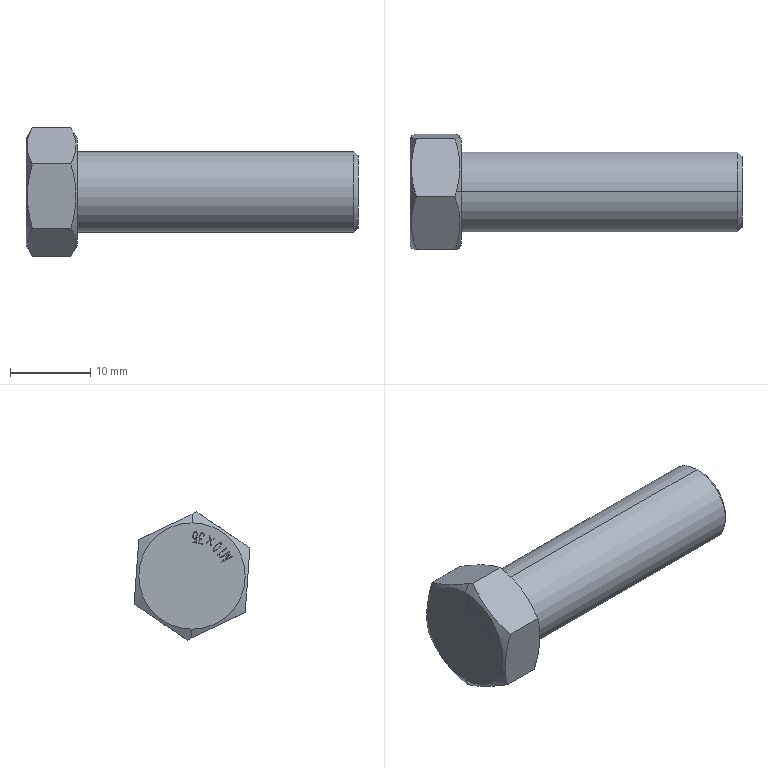Part | SolidWorks | features ICE 2, Chamfer 1, Extrusion 1, MirrorPattern 1, RevCut 1 | 1 solid | 146 faces | box 41.4 x 14.441 x 16 mm | volume 3801 mm3 | plane 89 | spline 49 | cone 6 | cylinder 2 | commonest cylinder face diameters 10 x2